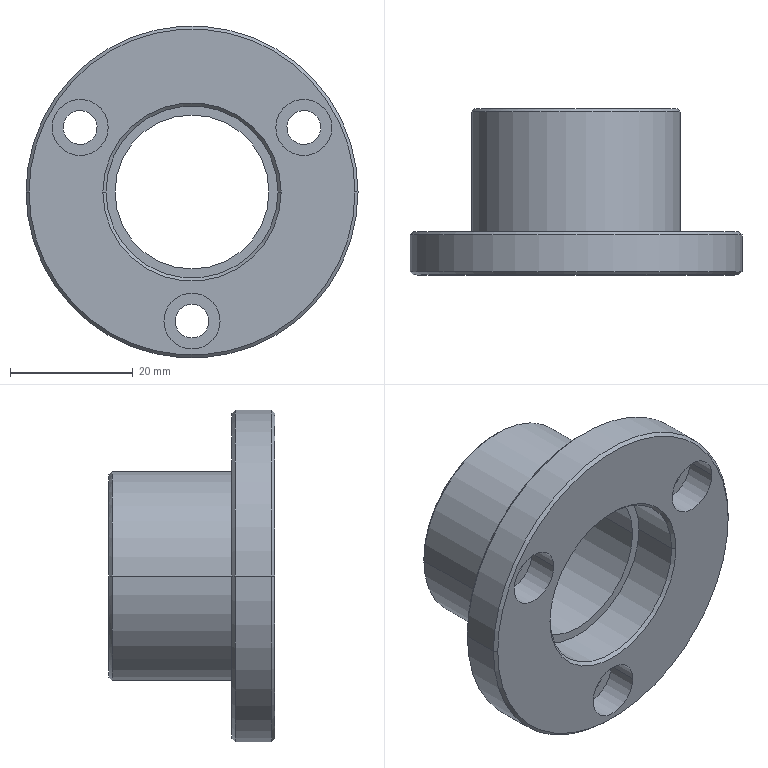Part | Creo | features CUT 4, CURVE 3, DATUM PLANE 3, CHAMFER 1, COORDINATE SYSTEM 1, PATTERN 1, PROTRUSION 1 | 1 solid | 40 faces | box 54 x 27 x 54 mm | volume 17717 mm3 | cylinder 22 | cone 10 | plane 8 | commonest cylinder face diameters 5.5 x6 9.13 x6 28 x4 25.045 x2 34 x2 54 x2
STEP:
#1=CARTESIAN_POINT('',(0.,0.,0.));
#2=DIRECTION('',(0.,0.,1.));
#3=DIRECTION('',(1.,0.,0.));
#4=AXIS2_PLACEMENT_3D('',#1,#2,#3);
#5=CARTESIAN_POINT('',(14.,0.5,0.));
#6=VERTEX_POINT('',#5);
#7=CARTESIAN_POINT('',(-14.,0.5,0.));
#8=VERTEX_POINT('',#7);
#9=CARTESIAN_POINT('',(0.,0.5,0.));
#10=DIRECTION('',(0.,1.,0.));
#11=DIRECTION('',(1.,0.,0.));
#12=AXIS2_PLACEMENT_3D('',#9,#10,#11);
#13=CIRCLE('',#12,14.);
#14=EDGE_CURVE('',#6,#8,#13,.T.);
#15=ORIENTED_EDGE('',*,*,#14,.T.);
#16=CARTESIAN_POINT('',(-14.,8.,0.));
#17=VERTEX_POINT('',#16);
#18=CARTESIAN_POINT('',(-14.,8.,0.));
#19=DIRECTION('',(0.,-1.,0.000000001));
#20=VECTOR('',#19,7.5);
#21=LINE('',#18,#20);
#22=EDGE_CURVE('',#17,#8,#21,.T.);
#23=ORIENTED_EDGE('',*,*,#22,.F.);
#24=CARTESIAN_POINT('',(14.,8.,0.));
#25=VERTEX_POINT('',#24);
#26=CARTESIAN_POINT('',(0.,8.,0.));
#27=DIRECTION('',(0.,1.,0.));
#28=DIRECTION('',(1.,0.,0.));
#29=AXIS2_PLACEMENT_3D('',#26,#27,#28);
#30=CIRCLE('',#29,14.);
#31=EDGE_CURVE('',#25,#17,#30,.T.);
#32=ORIENTED_EDGE('',*,*,#31,.F.);
#33=CARTESIAN_POINT('',(14.,8.,0.));
#34=DIRECTION('',(0.,-1.,-0.000000001));
#35=VECTOR('',#34,7.5);
#36=LINE('',#33,#35);
#37=EDGE_CURVE('',#25,#6,#36,.T.);
#38=ORIENTED_EDGE('',*,*,#37,.T.);
#39=EDGE_LOOP('',(#15,#23,#32,#38));
#40=FACE_OUTER_BOUND('',#39,.F.);
#41=CARTESIAN_POINT('',(0.,0.,0.));
#42=DIRECTION('',(0.,1.,0.));
#43=DIRECTION('',(1.,0.,0.));
#44=AXIS2_PLACEMENT_3D('',#41,#42,#43);
#45=CYLINDRICAL_SURFACE('',#44,14.);
#46=ADVANCED_FACE('',(#40),#45,.F.);
#47=CARTESIAN_POINT('',(14.5,0.,0.));
#48=VERTEX_POINT('',#47);
#49=CARTESIAN_POINT('',(-14.5,0.,0.));
#50=VERTEX_POINT('',#49);
#51=CARTESIAN_POINT('',(0.,0.,0.));
#52=DIRECTION('',(0.,1.,0.));
#53=DIRECTION('',(1.,0.,0.));
#54=AXIS2_PLACEMENT_3D('',#51,#52,#53);
#55=CIRCLE('',#54,14.5);
#56=EDGE_CURVE('',#48,#50,#55,.T.);
#57=ORIENTED_EDGE('',*,*,#56,.T.);
#58=CARTESIAN_POINT('',(-14.5,0.000000001,0.000000008));
#59=DIRECTION('',(0.7071,0.7071,-0.000000003));
#60=VECTOR('',#59,0.7071);
#61=LINE('',#58,#60);
#62=EDGE_CURVE('',#50,#8,#61,.T.);
#63=ORIENTED_EDGE('',*,*,#62,.T.);
#64=ORIENTED_EDGE('',*,*,#14,.F.);
#65=CARTESIAN_POINT('',(14.5,0.000000001,-0.000000008));
#66=DIRECTION('',(-0.7071,0.7071,0.000000003));
#67=VECTOR('',#66,0.7071);
#68=LINE('',#65,#67);
#69=EDGE_CURVE('',#48,#6,#68,.T.);
#70=ORIENTED_EDGE('',*,*,#69,.F.);
#71=EDGE_LOOP('',(#57,#63,#64,#70));
#72=FACE_OUTER_BOUND('',#71,.F.);
#73=CARTESIAN_POINT('',(0.,0.25,0.));
#74=DIRECTION('',(0.,-1.,0.));
#75=DIRECTION('',(0.,0.,-1.));
#76=AXIS2_PLACEMENT_3D('',#73,#74,#75);
#77=CONICAL_SURFACE('',#76,14.25,45.);
#78=ADVANCED_FACE('',(#72),#77,.F.);
#79=CARTESIAN_POINT('',(-26.5,0.,0.));
#80=VERTEX_POINT('',#79);
#81=CARTESIAN_POINT('',(26.5,0.,0.));
#82=VERTEX_POINT('',#81);
#83=CARTESIAN_POINT('',(0.,0.,0.));
#84=DIRECTION('',(0.,1.,0.));
#85=DIRECTION('',(-1.,0.,0.));
#86=AXIS2_PLACEMENT_3D('',#83,#84,#85);
#87=CIRCLE('',#86,26.5);
#88=EDGE_CURVE('',#80,#82,#87,.T.);
#89=ORIENTED_EDGE('',*,*,#88,.T.);
#90=CARTESIAN_POINT('',(0.,0.,0.));
#91=DIRECTION('',(0.,1.,0.));
#92=DIRECTION('',(1.,0.,0.));
#93=AXIS2_PLACEMENT_3D('',#90,#91,#92);
#94=CIRCLE('',#93,26.5);
#95=EDGE_CURVE('',#82,#80,#94,.T.);
#96=ORIENTED_EDGE('',*,*,#95,.T.);
#97=EDGE_LOOP('',(#89,#96));
#98=FACE_OUTER_BOUND('',#97,.F.);
#99=CARTESIAN_POINT('',(13.622,0.,10.5));
#100=VERTEX_POINT('',#99);
#101=CARTESIAN_POINT('',(22.751,0.,10.5));
#102=VERTEX_POINT('',#101);
#103=CARTESIAN_POINT('',(18.187,0.,10.5));
#104=DIRECTION('',(0.,-1.,0.));
#105=DIRECTION('',(-1.,0.,0.));
#106=AXIS2_PLACEMENT_3D('',#103,#104,#105);
#107=CIRCLE('',#106,4.565);
#108=EDGE_CURVE('',#100,#102,#107,.T.);
#109=ORIENTED_EDGE('',*,*,#108,.T.);
#110=CARTESIAN_POINT('',(18.187,0.,10.5));
#111=DIRECTION('',(0.,-1.,0.));
#112=DIRECTION('',(1.,0.,0.));
#113=AXIS2_PLACEMENT_3D('',#110,#111,#112);
#114=CIRCLE('',#113,4.565);
#115=EDGE_CURVE('',#102,#100,#114,.T.);
#116=ORIENTED_EDGE('',*,*,#115,.T.);
#117=EDGE_LOOP('',(#109,#116));
#118=FACE_BOUND('',#117,.F.);
#119=CARTESIAN_POINT('',(-22.751,0.,10.5));
#120=VERTEX_POINT('',#119);
#121=CARTESIAN_POINT('',(-13.622,0.,10.5));
#122=VERTEX_POINT('',#121);
#123=CARTESIAN_POINT('',(-18.187,0.,10.5));
#124=DIRECTION('',(0.,-1.,0.));
#125=DIRECTION('',(-1.,0.,0.));
#126=AXIS2_PLACEMENT_3D('',#123,#124,#125);
#127=CIRCLE('',#126,4.565);
#128=EDGE_CURVE('',#120,#122,#127,.T.);
#129=ORIENTED_EDGE('',*,*,#128,.T.);
#130=CARTESIAN_POINT('',(-18.187,0.,10.5));
#131=DIRECTION('',(0.,-1.,0.));
#132=DIRECTION('',(1.,0.,0.));
#133=AXIS2_PLACEMENT_3D('',#130,#131,#132);
#134=CIRCLE('',#133,4.565);
#135=EDGE_CURVE('',#122,#120,#134,.T.);
#136=ORIENTED_EDGE('',*,*,#135,.T.);
#137=EDGE_LOOP('',(#129,#136));
#138=FACE_BOUND('',#137,.F.);
#139=CARTESIAN_POINT('',(-4.565,0.,-21.));
#140=VERTEX_POINT('',#139);
#141=CARTESIAN_POINT('',(4.565,0.,-21.));
#142=VERTEX_POINT('',#141);
#143=CARTESIAN_POINT('',(0.,0.,-21.));
#144=DIRECTION('',(0.,-1.,0.));
#145=DIRECTION('',(-1.,0.,0.));
#146=AXIS2_PLACEMENT_3D('',#143,#144,#145);
#147=CIRCLE('',#146,4.565);
#148=EDGE_CURVE('',#140,#142,#147,.T.);
#149=ORIENTED_EDGE('',*,*,#148,.T.);
#150=CARTESIAN_POINT('',(0.,0.,-21.));
#151=DIRECTION('',(0.,-1.,0.));
#152=DIRECTION('',(1.,0.,0.));
#153=AXIS2_PLACEMENT_3D('',#150,#151,#152);
#154=CIRCLE('',#153,4.565);
#155=EDGE_CURVE('',#142,#140,#154,.T.);
#156=ORIENTED_EDGE('',*,*,#155,.T.);
#157=EDGE_LOOP('',(#149,#156));
#158=FACE_BOUND('',#157,.F.);
#159=CARTESIAN_POINT('',(0.,0.,0.));
#160=DIRECTION('',(0.,1.,0.));
#161=DIRECTION('',(-1.,0.,0.));
#162=AXIS2_PLACEMENT_3D('',#159,#160,#161);
#163=CIRCLE('',#162,14.5);
#164=EDGE_CURVE('',#50,#48,#163,.T.);
#165=ORIENTED_EDGE('',*,*,#164,.F.);
#166=ORIENTED_EDGE('',*,*,#56,.F.);
#167=EDGE_LOOP('',(#165,#166));
#168=FACE_BOUND('',#167,.F.);
#169=CARTESIAN_POINT('',(0.,0.,0.));
#170=DIRECTION('',(0.,1.,0.));
#171=DIRECTION('',(1.,0.,0.));
#172=AXIS2_PLACEMENT_3D('',#169,#170,#171);
#173=PLANE('',#172);
#174=ADVANCED_FACE('',(#98,#118,#138,#158,#168),#173,.F.);
#175=ORIENTED_EDGE('',*,*,#148,.F.);
#176=CARTESIAN_POINT('',(-4.565,5.,-21.));
#177=VERTEX_POINT('',#176);
#178=CARTESIAN_POINT('',(-4.565,0.,-21.));
#179=DIRECTION('',(0.,1.,0.));
#180=VECTOR('',#179,5.);
#181=LINE('',#178,#180);
#182=EDGE_CURVE('',#140,#177,#181,.T.);
#183=ORIENTED_EDGE('',*,*,#182,.T.);
#184=CARTESIAN_POINT('',(4.565,5.,-21.));
#185=VERTEX_POINT('',#184);
#186=CARTESIAN_POINT('',(0.,5.,-21.));
#187=DIRECTION('',(0.,-1.,0.));
#188=DIRECTION('',(-1.,0.,0.));
#189=AXIS2_PLACEMENT_3D('',#186,#187,#188);
#190=CIRCLE('',#189,4.565);
#191=EDGE_CURVE('',#177,#185,#190,.T.);
#192=ORIENTED_EDGE('',*,*,#191,.T.);
#193=CARTESIAN_POINT('',(4.565,0.,-21.));
#194=DIRECTION('',(0.,1.,0.));
#195=VECTOR('',#194,5.);
#196=LINE('',#193,#195);
#197=EDGE_CURVE('',#142,#185,#196,.T.);
#198=ORIENTED_EDGE('',*,*,#197,.F.);
#199=EDGE_LOOP('',(#175,#183,#192,#198));
#200=FACE_OUTER_BOUND('',#199,.F.);
#201=CARTESIAN_POINT('',(0.,0.,-21.));
#202=DIRECTION('',(0.,-1.,0.));
#203=DIRECTION('',(-1.,0.,0.));
#204=AXIS2_PLACEMENT_3D('',#201,#202,#203);
#205=CYLINDRICAL_SURFACE('',#204,4.565);
#206=ADVANCED_FACE('',(#200),#205,.F.);
#207=ORIENTED_EDGE('',*,*,#155,.F.);
#208=ORIENTED_EDGE('',*,*,#197,.T.);
#209=CARTESIAN_POINT('',(0.,5.,-21.));
#210=DIRECTION('',(0.,-1.,0.));
#211=DIRECTION('',(1.,0.,0.));
#212=AXIS2_PLACEMENT_3D('',#209,#210,#211);
#213=CIRCLE('',#212,4.565);
#214=EDGE_CURVE('',#185,#177,#213,.T.);
#215=ORIENTED_EDGE('',*,*,#214,.T.);
#216=ORIENTED_EDGE('',*,*,#182,.F.);
#217=EDGE_LOOP('',(#207,#208,#215,#216));
#218=FACE_OUTER_BOUND('',#217,.F.);
#219=CARTESIAN_POINT('',(0.,0.,-21.));
#220=DIRECTION('',(0.,-1.,0.));
#221=DIRECTION('',(-1.,0.,0.));
#222=AXIS2_PLACEMENT_3D('',#219,#220,#221);
#223=CYLINDRICAL_SURFACE('',#222,4.565);
#224=ADVANCED_FACE('',(#218),#223,.F.);
#225=ORIENTED_EDGE('',*,*,#191,.F.);
#226=ORIENTED_EDGE('',*,*,#214,.F.);
#227=EDGE_LOOP('',(#225,#226));
#228=FACE_OUTER_BOUND('',#227,.F.);
#229=CARTESIAN_POINT('',(2.75,5.,-21.));
#230=VERTEX_POINT('',#229);
#231=CARTESIAN_POINT('',(-2.75,5.,-21.));
#232=VERTEX_POINT('',#231);
#233=CARTESIAN_POINT('',(0.,5.,-21.));
#234=DIRECTION('',(0.,1.,0.));
#235=DIRECTION('',(1.,0.,0.));
#236=AXIS2_PLACEMENT_3D('',#233,#234,#235);
#237=CIRCLE('',#236,2.75);
#238=EDGE_CURVE('',#230,#232,#237,.T.);
#239=ORIENTED_EDGE('',*,*,#238,.F.);
#240=CARTESIAN_POINT('',(0.,5.,-21.));
#241=DIRECTION('',(0.,1.,0.));
#242=DIRECTION('',(-1.,0.,0.));
#243=AXIS2_PLACEMENT_3D('',#240,#241,#242);
#244=CIRCLE('',#243,2.75);
#245=EDGE_CURVE('',#232,#230,#244,.T.);
#246=ORIENTED_EDGE('',*,*,#245,.F.);
#247=EDGE_LOOP('',(#239,#246));
#248=FACE_BOUND('',#247,.F.);
#249=CARTESIAN_POINT('',(0.,5.,0.));
#250=DIRECTION('',(0.,-1.,0.));
#251=DIRECTION('',(-1.,0.,0.));
#252=AXIS2_PLACEMENT_3D('',#249,#250,#251);
#253=PLANE('',#252);
#254=ADVANCED_FACE('',(#228,#248),#253,.T.);
#255=CARTESIAN_POINT('',(13.622,5.,10.5));
#256=VERTEX_POINT('',#255);
#257=CARTESIAN_POINT('',(22.751,5.,10.5));
#258=VERTEX_POINT('',#257);
#259=CARTESIAN_POINT('',(18.187,5.,10.5));
#260=DIRECTION('',(0.,-1.,0.));
#261=DIRECTION('',(-1.,0.,0.));
#262=AXIS2_PLACEMENT_3D('',#259,#260,#261);
#263=CIRCLE('',#262,4.565);
#264=EDGE_CURVE('',#256,#258,#263,.T.);
#265=ORIENTED_EDGE('',*,*,#264,.F.);
#266=CARTESIAN_POINT('',(18.187,5.,10.5));
#267=DIRECTION('',(0.,-1.,0.));
#268=DIRECTION('',(1.,0.,0.));
#269=AXIS2_PLACEMENT_3D('',#266,#267,#268);
#270=CIRCLE('',#269,4.565);
#271=EDGE_CURVE('',#258,#256,#270,.T.);
#272=ORIENTED_EDGE('',*,*,#271,.F.);
#273=EDGE_LOOP('',(#265,#272));
#274=FACE_OUTER_BOUND('',#273,.F.);
#275=CARTESIAN_POINT('',(16.812,5.,12.882));
#276=VERTEX_POINT('',#275);
#277=CARTESIAN_POINT('',(19.562,5.,8.118));
#278=VERTEX_POINT('',#277);
#279=CARTESIAN_POINT('',(18.187,5.,10.5));
#280=DIRECTION('',(0.,1.,0.));
#281=DIRECTION('',(-0.5,0.,0.866));
#282=AXIS2_PLACEMENT_3D('',#279,#280,#281);
#283=CIRCLE('',#282,2.75);
#284=EDGE_CURVE('',#276,#278,#283,.T.);
#285=ORIENTED_EDGE('',*,*,#284,.F.);
#286=CARTESIAN_POINT('',(18.187,5.,10.5));
#287=DIRECTION('',(0.,1.,0.));
#288=DIRECTION('',(0.5,0.,-0.866));
#289=AXIS2_PLACEMENT_3D('',#286,#287,#288);
#290=CIRCLE('',#289,2.75);
#291=EDGE_CURVE('',#278,#276,#290,.T.);
#292=ORIENTED_EDGE('',*,*,#291,.F.);
#293=EDGE_LOOP('',(#285,#292));
#294=FACE_BOUND('',#293,.F.);
#295=CARTESIAN_POINT('',(0.,5.,0.));
#296=DIRECTION('',(0.,-1.,0.));
#297=DIRECTION('',(-1.,0.,0.));
#298=AXIS2_PLACEMENT_3D('',#295,#296,#297);
#299=PLANE('',#298);
#300=ADVANCED_FACE('',(#274,#294),#299,.T.);
#301=CARTESIAN_POINT('',(-22.751,5.,10.5));
#302=VERTEX_POINT('',#301);
#303=CARTESIAN_POINT('',(-13.622,5.,10.5));
#304=VERTEX_POINT('',#303);
#305=CARTESIAN_POINT('',(-18.187,5.,10.5));
#306=DIRECTION('',(0.,-1.,0.));
#307=DIRECTION('',(-1.,0.,0.));
#308=AXIS2_PLACEMENT_3D('',#305,#306,#307);
#309=CIRCLE('',#308,4.565);
#310=EDGE_CURVE('',#302,#304,#309,.T.);
#311=ORIENTED_EDGE('',*,*,#310,.F.);
#312=CARTESIAN_POINT('',(-18.187,5.,10.5));
#313=DIRECTION('',(0.,-1.,0.));
#314=DIRECTION('',(1.,0.,0.));
#315=AXIS2_PLACEMENT_3D('',#312,#313,#314);
#316=CIRCLE('',#315,4.565);
#317=EDGE_CURVE('',#304,#302,#316,.T.);
#318=ORIENTED_EDGE('',*,*,#317,.F.);
#319=EDGE_LOOP('',(#311,#318));
#320=FACE_OUTER_BOUND('',#319,.F.);
#321=CARTESIAN_POINT('',(-19.562,5.,8.118));
#322=VERTEX_POINT('',#321);
#323=CARTESIAN_POINT('',(-16.812,5.,12.882));
#324=VERTEX_POINT('',#323);
#325=CARTESIAN_POINT('',(-18.187,5.,10.5));
#326=DIRECTION('',(0.,1.,0.));
#327=DIRECTION('',(-0.5,0.,-0.866));
#328=AXIS2_PLACEMENT_3D('',#325,#326,#327);
#329=CIRCLE('',#328,2.75);
#330=EDGE_CURVE('',#322,#324,#329,.T.);
#331=ORIENTED_EDGE('',*,*,#330,.F.);
#332=CARTESIAN_POINT('',(-18.187,5.,10.5));
#333=DIRECTION('',(0.,1.,0.));
#334=DIRECTION('',(0.5,0.,0.866));
#335=AXIS2_PLACEMENT_3D('',#332,#333,#334);
#336=CIRCLE('',#335,2.75);
#337=EDGE_CURVE('',#324,#322,#336,.T.);
#338=ORIENTED_EDGE('',*,*,#337,.F.);
#339=EDGE_LOOP('',(#331,#338));
#340=FACE_BOUND('',#339,.F.);
#341=CARTESIAN_POINT('',(0.,5.,0.));
#342=DIRECTION('',(0.,-1.,0.));
#343=DIRECTION('',(-1.,0.,0.));
#344=AXIS2_PLACEMENT_3D('',#341,#342,#343);
#345=PLANE('',#344);
#346=ADVANCED_FACE('',(#320,#340),#345,.T.);
#347=ORIENTED_EDGE('',*,*,#108,.F.);
#348=CARTESIAN_POINT('',(13.622,0.,10.5));
#349=DIRECTION('',(0.,1.,0.));
#350=VECTOR('',#349,5.);
#351=LINE('',#348,#350);
#352=EDGE_CURVE('',#100,#256,#351,.T.);
#353=ORIENTED_EDGE('',*,*,#352,.T.);
#354=ORIENTED_EDGE('',*,*,#264,.T.);
#355=CARTESIAN_POINT('',(22.751,0.,10.5));
#356=DIRECTION('',(0.,1.,0.));
#357=VECTOR('',#356,5.);
#358=LINE('',#355,#357);
#359=EDGE_CURVE('',#102,#258,#358,.T.);
#360=ORIENTED_EDGE('',*,*,#359,.F.);
#361=EDGE_LOOP('',(#347,#353,#354,#360));
#362=FACE_OUTER_BOUND('',#361,.F.);
#363=CARTESIAN_POINT('',(18.187,0.,10.5));
#364=DIRECTION('',(0.,-1.,0.));
#365=DIRECTION('',(-1.,0.,0.));
#366=AXIS2_PLACEMENT_3D('',#363,#364,#365);
#367=CYLINDRICAL_SURFACE('',#366,4.565);
#368=ADVANCED_FACE('',(#362),#367,.F.);
#369=ORIENTED_EDGE('',*,*,#115,.F.);
#370=ORIENTED_EDGE('',*,*,#359,.T.);
#371=ORIENTED_EDGE('',*,*,#271,.T.);
#372=ORIENTED_EDGE('',*,*,#352,.F.);
#373=EDGE_LOOP('',(#369,#370,#371,#372));
#374=FACE_OUTER_BOUND('',#373,.F.);
#375=CARTESIAN_POINT('',(18.187,0.,10.5));
#376=DIRECTION('',(0.,-1.,0.));
#377=DIRECTION('',(-1.,0.,0.));
#378=AXIS2_PLACEMENT_3D('',#375,#376,#377);
#379=CYLINDRICAL_SURFACE('',#378,4.565);
#380=ADVANCED_FACE('',(#374),#379,.F.);
#381=ORIENTED_EDGE('',*,*,#128,.F.);
#382=CARTESIAN_POINT('',(-22.751,0.,10.5));
#383=DIRECTION('',(0.,1.,0.));
#384=VECTOR('',#383,5.);
#385=LINE('',#382,#384);
#386=EDGE_CURVE('',#120,#302,#385,.T.);
#387=ORIENTED_EDGE('',*,*,#386,.T.);
#388=ORIENTED_EDGE('',*,*,#310,.T.);
#389=CARTESIAN_POINT('',(-13.622,0.,10.5));
#390=DIRECTION('',(0.,1.,0.));
#391=VECTOR('',#390,5.);
#392=LINE('',#389,#391);
#393=EDGE_CURVE('',#122,#304,#392,.T.);
#394=ORIENTED_EDGE('',*,*,#393,.F.);
#395=EDGE_LOOP('',(#381,#387,#388,#394));
#396=FACE_OUTER_BOUND('',#395,.F.);
#397=CARTESIAN_POINT('',(-18.187,0.,10.5));
#398=DIRECTION('',(0.,-1.,0.));
#399=DIRECTION('',(-1.,0.,0.));
#400=AXIS2_PLACEMENT_3D('',#397,#398,#399);
#401=CYLINDRICAL_SURFACE('',#400,4.565);
#402=ADVANCED_FACE('',(#396),#401,.F.);
#403=ORIENTED_EDGE('',*,*,#135,.F.);
#404=ORIENTED_EDGE('',*,*,#393,.T.);
#405=ORIENTED_EDGE('',*,*,#317,.T.);
#406=ORIENTED_EDGE('',*,*,#386,.F.);
#407=EDGE_LOOP('',(#403,#404,#405,#406));
#408=FACE_OUTER_BOUND('',#407,.F.);
#409=CARTESIAN_POINT('',(-18.187,0.,10.5));
#410=DIRECTION('',(0.,-1.,0.));
#411=DIRECTION('',(-1.,0.,0.));
#412=AXIS2_PLACEMENT_3D('',#409,#410,#411);
#413=CYLINDRICAL_SURFACE('',#412,4.565);
#414=ADVANCED_FACE('',(#408),#413,.F.);
#415=ORIENTED_EDGE('',*,*,#238,.T.);
#416=CARTESIAN_POINT('',(-2.75,7.,-21.));
#417=VERTEX_POINT('',#416);
#418=CARTESIAN_POINT('',(-2.75,7.,-21.));
#419=DIRECTION('',(0.,-1.,0.));
#420=VECTOR('',#419,2.);
#421=LINE('',#418,#420);
#422=EDGE_CURVE('',#417,#232,#421,.T.);
#423=ORIENTED_EDGE('',*,*,#422,.F.);
#424=CARTESIAN_POINT('',(2.75,7.,-21.));
#425=VERTEX_POINT('',#424);
#426=CARTESIAN_POINT('',(0.,7.,-21.));
#427=DIRECTION('',(0.,1.,0.));
#428=DIRECTION('',(1.,0.,0.));
#429=AXIS2_PLACEMENT_3D('',#426,#427,#428);
#430=CIRCLE('',#429,2.75);
#431=EDGE_CURVE('',#425,#417,#430,.T.);
#432=ORIENTED_EDGE('',*,*,#431,.F.);
#433=CARTESIAN_POINT('',(2.75,7.,-21.));
#434=DIRECTION('',(0.,-1.,0.));
#435=VECTOR('',#434,2.);
#436=LINE('',#433,#435);
#437=EDGE_CURVE('',#425,#230,#436,.T.);
#438=ORIENTED_EDGE('',*,*,#437,.T.);
#439=EDGE_LOOP('',(#415,#423,#432,#438));
#440=FACE_OUTER_BOUND('',#439,.F.);
#441=CARTESIAN_POINT('',(0.,7.,-21.));
#442=DIRECTION('',(0.,1.,0.));
#443=DIRECTION('',(1.,0.,0.));
#444=AXIS2_PLACEMENT_3D('',#441,#442,#443);
#445=CYLINDRICAL_SURFACE('',#444,2.75);
#446=ADVANCED_FACE('',(#440),#445,.F.);
#447=ORIENTED_EDGE('',*,*,#245,.T.);
#448=ORIENTED_EDGE('',*,*,#437,.F.);
#449=CARTESIAN_POINT('',(0.,7.,-21.));
#450=DIRECTION('',(0.,1.,0.));
#451=DIRECTION('',(-1.,0.,0.));
#452=AXIS2_PLACEMENT_3D('',#449,#450,#451);
#453=CIRCLE('',#452,2.75);
#454=EDGE_CURVE('',#417,#425,#453,.T.);
#455=ORIENTED_EDGE('',*,*,#454,.F.);
#456=ORIENTED_EDGE('',*,*,#422,.T.);
#457=EDGE_LOOP('',(#447,#448,#455,#456));
#458=FACE_OUTER_BOUND('',#457,.F.);
#459=CARTESIAN_POINT('',(0.,7.,-21.));
#460=DIRECTION('',(0.,1.,0.));
#461=DIRECTION('',(1.,0.,0.));
#462=AXIS2_PLACEMENT_3D('',#459,#460,#461);
#463=CYLINDRICAL_SURFACE('',#462,2.75);
#464=ADVANCED_FACE('',(#458),#463,.F.);
#465=CARTESIAN_POINT('',(-26.5,7.,0.));
#466=VERTEX_POINT('',#465);
#467=CARTESIAN_POINT('',(26.5,7.,0.));
#468=VERTEX_POINT('',#467);
#469=CARTESIAN_POINT('',(0.,7.,0.));
#470=DIRECTION('',(0.,1.,0.));
#471=DIRECTION('',(-1.,0.,0.));
#472=AXIS2_PLACEMENT_3D('',#469,#470,#471);
#473=CIRCLE('',#472,26.5);
#474=EDGE_CURVE('',#466,#468,#473,.T.);
#475=ORIENTED_EDGE('',*,*,#474,.F.);
#476=CARTESIAN_POINT('',(0.,7.,0.));
#477=DIRECTION('',(0.,1.,0.));
#478=DIRECTION('',(1.,0.,0.));
#479=AXIS2_PLACEMENT_3D('',#476,#477,#478);
#480=CIRCLE('',#479,26.5);
#481=EDGE_CURVE('',#468,#466,#480,.T.);
#482=ORIENTED_EDGE('',*,*,#481,.F.);
#483=EDGE_LOOP('',(#475,#482));
#484=FACE_OUTER_BOUND('',#483,.F.);
#485=ORIENTED_EDGE('',*,*,#431,.T.);
#486=ORIENTED_EDGE('',*,*,#454,.T.);
#487=EDGE_LOOP('',(#485,#486));
#488=FACE_BOUND('',#487,.F.);
#489=CARTESIAN_POINT('',(-19.562,7.,8.118));
#490=VERTEX_POINT('',#489);
#491=CARTESIAN_POINT('',(-16.812,7.,12.882));
#492=VERTEX_POINT('',#491);
#493=CARTESIAN_POINT('',(-18.187,7.,10.5));
#494=DIRECTION('',(0.,1.,0.));
#495=DIRECTION('',(-0.5,0.,-0.866));
#496=AXIS2_PLACEMENT_3D('',#493,#494,#495);
#497=CIRCLE('',#496,2.75);
#498=EDGE_CURVE('',#490,#492,#497,.T.);
#499=ORIENTED_EDGE('',*,*,#498,.T.);
#500=CARTESIAN_POINT('',(-18.187,7.,10.5));
#501=DIRECTION('',(0.,1.,0.));
#502=DIRECTION('',(0.5,0.,0.866));
#503=AXIS2_PLACEMENT_3D('',#500,#501,#502);
#504=CIRCLE('',#503,2.75);
#505=EDGE_CURVE('',#492,#490,#504,.T.);
#506=ORIENTED_EDGE('',*,*,#505,.T.);
#507=EDGE_LOOP('',(#499,#506));
#508=FACE_BOUND('',#507,.F.);
#509=CARTESIAN_POINT('',(16.812,7.,12.882));
#510=VERTEX_POINT('',#509);
#511=CARTESIAN_POINT('',(19.562,7.,8.118));
#512=VERTEX_POINT('',#511);
#513=CARTESIAN_POINT('',(18.187,7.,10.5));
#514=DIRECTION('',(0.,1.,0.));
#515=DIRECTION('',(-0.5,0.,0.866));
#516=AXIS2_PLACEMENT_3D('',#513,#514,#515);
#517=CIRCLE('',#516,2.75);
#518=EDGE_CURVE('',#510,#512,#517,.T.);
#519=ORIENTED_EDGE('',*,*,#518,.T.);
#520=CARTESIAN_POINT('',(18.187,7.,10.5));
#521=DIRECTION('',(0.,1.,0.));
#522=DIRECTION('',(0.5,0.,-0.866));
#523=AXIS2_PLACEMENT_3D('',#520,#521,#522);
#524=CIRCLE('',#523,2.75);
#525=EDGE_CURVE('',#512,#510,#524,.T.);
#526=ORIENTED_EDGE('',*,*,#525,.T.);
#527=EDGE_LOOP('',(#519,#526));
#528=FACE_BOUND('',#527,.F.);
#529=CARTESIAN_POINT('',(17.,7.,0.));
#530=VERTEX_POINT('',#529);
#531=CARTESIAN_POINT('',(-17.,7.,0.));
#532=VERTEX_POINT('',#531);
#533=CARTESIAN_POINT('',(0.,7.,0.));
#534=DIRECTION('',(0.,-1.,0.));
#535=DIRECTION('',(1.,0.,0.));
#536=AXIS2_PLACEMENT_3D('',#533,#534,#535);
#537=CIRCLE('',#536,17.);
#538=EDGE_CURVE('',#530,#532,#537,.T.);
#539=ORIENTED_EDGE('',*,*,#538,.F.);
#540=CARTESIAN_POINT('',(0.,7.,0.));
#541=DIRECTION('',(0.,1.,0.));
#542=DIRECTION('',(1.,0.,0.));
#543=AXIS2_PLACEMENT_3D('',#540,#541,#542);
#544=CIRCLE('',#543,17.);
#545=EDGE_CURVE('',#530,#532,#544,.T.);
#546=ORIENTED_EDGE('',*,*,#545,.T.);
#547=EDGE_LOOP('',(#539,#546));
#548=FACE_BOUND('',#547,.F.);
#549=CARTESIAN_POINT('',(0.,7.,0.));
#550=DIRECTION('',(0.,1.,0.));
#551=DIRECTION('',(1.,0.,0.));
#552=AXIS2_PLACEMENT_3D('',#549,#550,#551);
#553=PLANE('',#552);
#554=ADVANCED_FACE('',(#484,#488,#508,#528,#548),#553,.T.);
#555=CARTESIAN_POINT('',(-17.,26.5,0.));
#556=VERTEX_POINT('',#555);
#557=CARTESIAN_POINT('',(17.,26.5,0.));
#558=VERTEX_POINT('',#557);
#559=CARTESIAN_POINT('',(0.,26.5,0.));
#560=DIRECTION('',(0.,1.,0.));
#561=DIRECTION('',(-1.,0.,0.));
#562=AXIS2_PLACEMENT_3D('',#559,#560,#561);
#563=CIRCLE('',#562,17.);
#564=EDGE_CURVE('',#556,#558,#563,.T.);
#565=ORIENTED_EDGE('',*,*,#564,.T.);
#566=CARTESIAN_POINT('',(17.,7.,0.));
#567=DIRECTION('',(0.,1.,0.));
#568=VECTOR('',#567,19.5);
#569=LINE('',#566,#568);
#570=EDGE_CURVE('',#530,#558,#569,.T.);
#571=ORIENTED_EDGE('',*,*,#570,.F.);
#572=ORIENTED_EDGE('',*,*,#538,.T.);
#573=CARTESIAN_POINT('',(-17.,7.,0.));
#574=DIRECTION('',(0.,1.,0.));
#575=VECTOR('',#574,19.5);
#576=LINE('',#573,#575);
#577=EDGE_CURVE('',#532,#556,#576,.T.);
#578=ORIENTED_EDGE('',*,*,#577,.T.);
#579=EDGE_LOOP('',(#565,#571,#572,#578));
#580=FACE_OUTER_BOUND('',#579,.F.);
#581=CARTESIAN_POINT('',(0.,0.,0.));
#582=DIRECTION('',(0.,1.,0.));
#583=DIRECTION('',(1.,0.,0.));
#584=AXIS2_PLACEMENT_3D('',#581,#582,#583);
#585=CYLINDRICAL_SURFACE('',#584,17.);
#586=ADVANCED_FACE('',(#580),#585,.T.);
#587=CARTESIAN_POINT('',(-16.5,27.,0.));
#588=VERTEX_POINT('',#587);
#589=CARTESIAN_POINT('',(16.5,27.,0.));
#590=VERTEX_POINT('',#589);
#591=CARTESIAN_POINT('',(0.,27.,0.));
#592=DIRECTION('',(0.,1.,0.));
#593=DIRECTION('',(-1.,0.,0.));
#594=AXIS2_PLACEMENT_3D('',#591,#592,#593);
#595=CIRCLE('',#594,16.5);
#596=EDGE_CURVE('',#588,#590,#595,.T.);
#597=ORIENTED_EDGE('',*,*,#596,.T.);
#598=CARTESIAN_POINT('',(16.5,27.,-0.000000005));
#599=DIRECTION('',(0.7071,-0.7071,0.000000001));
#600=VECTOR('',#599,0.7071);
#601=LINE('',#598,#600);
#602=EDGE_CURVE('',#590,#558,#601,.T.);
#603=ORIENTED_EDGE('',*,*,#602,.T.);
#604=ORIENTED_EDGE('',*,*,#564,.F.);
#605=CARTESIAN_POINT('',(-16.5,27.,0.000000005));
#606=DIRECTION('',(-0.7071,-0.7071,-0.000000001));
#607=VECTOR('',#606,0.7071);
#608=LINE('',#605,#607);
#609=EDGE_CURVE('',#588,#556,#608,.T.);
#610=ORIENTED_EDGE('',*,*,#609,.F.);
#611=EDGE_LOOP('',(#597,#603,#604,#610));
#612=FACE_OUTER_BOUND('',#611,.F.);
#613=CARTESIAN_POINT('',(0.,26.75,0.));
#614=DIRECTION('',(0.,-1.,0.));
#615=DIRECTION('',(0.,0.,-1.));
#616=AXIS2_PLACEMENT_3D('',#613,#614,#615);
#617=CONICAL_SURFACE('',#616,16.75,45.);
#618=ADVANCED_FACE('',(#612),#617,.T.);
#619=ORIENTED_EDGE('',*,*,#596,.F.);
#620=CARTESIAN_POINT('',(0.,27.,0.));
#621=DIRECTION('',(0.,1.,0.));
#622=DIRECTION('',(1.,0.,0.));
#623=AXIS2_PLACEMENT_3D('',#620,#621,#622);
#624=CIRCLE('',#623,16.5);
#625=EDGE_CURVE('',#590,#588,#624,.T.);
#626=ORIENTED_EDGE('',*,*,#625,.F.);
#627=EDGE_LOOP('',(#619,#626));
#628=FACE_OUTER_BOUND('',#627,.F.);
#629=CARTESIAN_POINT('',(-14.5,27.,0.));
#630=VERTEX_POINT('',#629);
#631=CARTESIAN_POINT('',(14.5,27.,0.));
#632=VERTEX_POINT('',#631);
#633=CARTESIAN_POINT('',(0.,27.,0.));
#634=DIRECTION('',(0.,1.,0.));
#635=DIRECTION('',(-1.,0.,0.));
#636=AXIS2_PLACEMENT_3D('',#633,#634,#635);
#637=CIRCLE('',#636,14.5);
#638=EDGE_CURVE('',#630,#632,#637,.T.);
#639=ORIENTED_EDGE('',*,*,#638,.T.);
#640=CARTESIAN_POINT('',(0.,27.,0.));
#641=DIRECTION('',(0.,1.,0.));
#642=DIRECTION('',(1.,0.,0.));
#643=AXIS2_PLACEMENT_3D('',#640,#641,#642);
#644=CIRCLE('',#643,14.5);
#645=EDGE_CURVE('',#632,#630,#644,.T.);
#646=ORIENTED_EDGE('',*,*,#645,.T.);
#647=EDGE_LOOP('',(#639,#646));
#648=FACE_BOUND('',#647,.F.);
#649=CARTESIAN_POINT('',(0.,27.,0.));
#650=DIRECTION('',(0.,1.,0.));
#651=DIRECTION('',(1.,0.,0.));
#652=AXIS2_PLACEMENT_3D('',#649,#650,#651);
#653=PLANE('',#652);
#654=ADVANCED_FACE('',(#628,#648),#653,.T.);
#655=ORIENTED_EDGE('',*,*,#625,.T.);
#656=ORIENTED_EDGE('',*,*,#609,.T.);
#657=CARTESIAN_POINT('',(0.,26.5,0.));
#658=DIRECTION('',(0.,1.,0.));
#659=DIRECTION('',(1.,0.,0.));
#660=AXIS2_PLACEMENT_3D('',#657,#658,#659);
#661=CIRCLE('',#660,17.);
#662=EDGE_CURVE('',#558,#556,#661,.T.);
#663=ORIENTED_EDGE('',*,*,#662,.F.);
#664=ORIENTED_EDGE('',*,*,#602,.F.);
#665=EDGE_LOOP('',(#655,#656,#663,#664));
#666=FACE_OUTER_BOUND('',#665,.F.);
#667=CARTESIAN_POINT('',(0.,26.75,0.));
#668=DIRECTION('',(0.,-1.,0.));
#669=DIRECTION('',(0.,0.,-1.));
#670=AXIS2_PLACEMENT_3D('',#667,#668,#669);
#671=CONICAL_SURFACE('',#670,16.75,45.);
#672=ADVANCED_FACE('',(#666),#671,.T.);
#673=ORIENTED_EDGE('',*,*,#662,.T.);
#674=ORIENTED_EDGE('',*,*,#577,.F.);
#675=ORIENTED_EDGE('',*,*,#545,.F.);
#676=ORIENTED_EDGE('',*,*,#570,.T.);
#677=EDGE_LOOP('',(#673,#674,#675,#676));
#678=FACE_OUTER_BOUND('',#677,.F.);
#679=CARTESIAN_POINT('',(0.,0.,0.));
#680=DIRECTION('',(0.,1.,0.));
#681=DIRECTION('',(1.,0.,0.));
#682=AXIS2_PLACEMENT_3D('',#679,#680,#681);
#683=CYLINDRICAL_SURFACE('',#682,17.);
#684=ADVANCED_FACE('',(#678),#683,.T.);
#685=CARTESIAN_POINT('',(-14.,26.5,0.));
#686=VERTEX_POINT('',#685);
#687=CARTESIAN_POINT('',(14.,26.5,0.));
#688=VERTEX_POINT('',#687);
#689=CARTESIAN_POINT('',(0.,26.5,0.));
#690=DIRECTION('',(0.,1.,0.));
#691=DIRECTION('',(-1.,0.,0.));
#692=AXIS2_PLACEMENT_3D('',#689,#690,#691);
#693=CIRCLE('',#692,14.);
#694=EDGE_CURVE('',#686,#688,#693,.T.);
#695=ORIENTED_EDGE('',*,*,#694,.T.);
#696=CARTESIAN_POINT('',(14.,26.5,0.000000002));
#697=DIRECTION('',(0.7071,0.7071,0.000000001));
#698=VECTOR('',#697,0.7071);
#699=LINE('',#696,#698);
#700=EDGE_CURVE('',#688,#632,#699,.T.);
#701=ORIENTED_EDGE('',*,*,#700,.T.);
#702=ORIENTED_EDGE('',*,*,#638,.F.);
#703=CARTESIAN_POINT('',(-14.,26.5,-0.000000002));
#704=DIRECTION('',(-0.7071,0.7071,-0.000000001));
#705=VECTOR('',#704,0.7071);
#706=LINE('',#703,#705);
#707=EDGE_CURVE('',#686,#630,#706,.T.);
#708=ORIENTED_EDGE('',*,*,#707,.F.);
#709=EDGE_LOOP('',(#695,#701,#702,#708));
#710=FACE_OUTER_BOUND('',#709,.F.);
#711=CARTESIAN_POINT('',(0.,26.75,0.));
#712=DIRECTION('',(0.,1.,0.));
#713=DIRECTION('',(0.,0.,-1.));
#714=AXIS2_PLACEMENT_3D('',#711,#712,#713);
#715=CONICAL_SURFACE('',#714,14.25,45.);
#716=ADVANCED_FACE('',(#710),#715,.F.);
#717=ORIENTED_EDGE('',*,*,#694,.F.);
#718=CARTESIAN_POINT('',(-14.,19.,0.));
#719=VERTEX_POINT('',#718);
#720=CARTESIAN_POINT('',(-14.,26.5,-0.000000002));
#721=DIRECTION('',(0.,-1.,0.));
#722=VECTOR('',#721,7.5);
#723=LINE('',#720,#722);
#724=EDGE_CURVE('',#686,#719,#723,.T.);
#725=ORIENTED_EDGE('',*,*,#724,.T.);
#726=CARTESIAN_POINT('',(14.,19.,0.));
#727=VERTEX_POINT('',#726);
#728=CARTESIAN_POINT('',(0.,19.,0.));
#729=DIRECTION('',(0.,-1.,0.));
#730=DIRECTION('',(1.,0.,0.));
#731=AXIS2_PLACEMENT_3D('',#728,#729,#730);
#732=CIRCLE('',#731,14.);
#733=EDGE_CURVE('',#727,#719,#732,.T.);
#734=ORIENTED_EDGE('',*,*,#733,.F.);
#735=CARTESIAN_POINT('',(14.,26.5,0.000000002));
#736=DIRECTION('',(0.,-1.,0.));
#737=VECTOR('',#736,7.5);
#738=LINE('',#735,#737);
#739=EDGE_CURVE('',#688,#727,#738,.T.);
#740=ORIENTED_EDGE('',*,*,#739,.F.);
#741=EDGE_LOOP('',(#717,#725,#734,#740));
#742=FACE_OUTER_BOUND('',#741,.F.);
#743=CARTESIAN_POINT('',(0.,0.,0.));
#744=DIRECTION('',(0.,1.,0.));
#745=DIRECTION('',(1.,0.,0.));
#746=AXIS2_PLACEMENT_3D('',#743,#744,#745);
#747=CYLINDRICAL_SURFACE('',#746,14.);
#748=ADVANCED_FACE('',(#742),#747,.F.);
#749=CARTESIAN_POINT('',(0.,26.5,0.));
#750=DIRECTION('',(0.,1.,0.));
#751=DIRECTION('',(1.,0.,0.));
#752=AXIS2_PLACEMENT_3D('',#749,#750,#751);
#753=CIRCLE('',#752,14.);
#754=EDGE_CURVE('',#688,#686,#753,.T.);
#755=ORIENTED_EDGE('',*,*,#754,.F.);
#756=ORIENTED_EDGE('',*,*,#739,.T.);
#757=CARTESIAN_POINT('',(0.,19.,0.));
#758=DIRECTION('',(0.,1.,0.));
#759=DIRECTION('',(1.,0.,0.));
#760=AXIS2_PLACEMENT_3D('',#757,#758,#759);
#761=CIRCLE('',#760,14.);
#762=EDGE_CURVE('',#727,#719,#761,.T.);
#763=ORIENTED_EDGE('',*,*,#762,.T.);
#764=ORIENTED_EDGE('',*,*,#724,.F.);
#765=EDGE_LOOP('',(#755,#756,#763,#764));
#766=FACE_OUTER_BOUND('',#765,.F.);
#767=CARTESIAN_POINT('',(0.,0.,0.));
#768=DIRECTION('',(0.,1.,0.));
#769=DIRECTION('',(1.,0.,0.));
#770=AXIS2_PLACEMENT_3D('',#767,#768,#769);
#771=CYLINDRICAL_SURFACE('',#770,14.);
#772=ADVANCED_FACE('',(#766),#771,.F.);
#773=ORIENTED_EDGE('',*,*,#754,.T.);
#774=ORIENTED_EDGE('',*,*,#707,.T.);
#775=ORIENTED_EDGE('',*,*,#645,.F.);
#776=ORIENTED_EDGE('',*,*,#700,.F.);
#777=EDGE_LOOP('',(#773,#774,#775,#776));
#778=FACE_OUTER_BOUND('',#777,.F.);
#779=CARTESIAN_POINT('',(0.,26.75,0.));
#780=DIRECTION('',(0.,1.,0.));
#781=DIRECTION('',(0.,0.,-1.));
#782=AXIS2_PLACEMENT_3D('',#779,#780,#781);
#783=CONICAL_SURFACE('',#782,14.25,45.);
#784=ADVANCED_FACE('',(#778),#783,.F.);
#785=ORIENTED_EDGE('',*,*,#762,.F.);
#786=ORIENTED_EDGE('',*,*,#733,.T.);
#787=EDGE_LOOP('',(#785,#786));
#788=FACE_OUTER_BOUND('',#787,.F.);
#789=CARTESIAN_POINT('',(12.522,19.,0.));
#790=VERTEX_POINT('',#789);
#791=CARTESIAN_POINT('',(-12.522,19.,0.));
#792=VERTEX_POINT('',#791);
#793=CARTESIAN_POINT('',(0.,19.,0.));
#794=DIRECTION('',(0.,-1.,0.));
#795=DIRECTION('',(1.,0.,0.));
#796=AXIS2_PLACEMENT_3D('',#793,#794,#795);
#797=CIRCLE('',#796,12.522);
#798=EDGE_CURVE('',#790,#792,#797,.T.);
#799=ORIENTED_EDGE('',*,*,#798,.F.);
#800=CARTESIAN_POINT('',(0.,19.,0.));
#801=DIRECTION('',(0.,1.,0.));
#802=DIRECTION('',(1.,0.,0.));
#803=AXIS2_PLACEMENT_3D('',#800,#801,#802);
#804=CIRCLE('',#803,12.522);
#805=EDGE_CURVE('',#790,#792,#804,.T.);
#806=ORIENTED_EDGE('',*,*,#805,.T.);
#807=EDGE_LOOP('',(#799,#806));
#808=FACE_BOUND('',#807,.F.);
#809=CARTESIAN_POINT('',(0.,19.,0.));
#810=DIRECTION('',(0.,1.,0.));
#811=DIRECTION('',(1.,0.,0.));
#812=AXIS2_PLACEMENT_3D('',#809,#810,#811);
#813=PLANE('',#812);
#814=ADVANCED_FACE('',(#788,#808),#813,.T.);
#815=CARTESIAN_POINT('',(12.522,8.,0.));
#816=VERTEX_POINT('',#815);
#817=CARTESIAN_POINT('',(12.522,19.,0.));
#818=DIRECTION('',(0.,-1.,0.));
#819=VECTOR('',#818,11.);
#820=LINE('',#817,#819);
#821=EDGE_CURVE('',#790,#816,#820,.T.);
#822=ORIENTED_EDGE('',*,*,#821,.F.);
#823=ORIENTED_EDGE('',*,*,#798,.T.);
#824=CARTESIAN_POINT('',(-12.522,8.,0.));
#825=VERTEX_POINT('',#824);
#826=CARTESIAN_POINT('',(-12.522,19.,0.));
#827=DIRECTION('',(0.,-1.,0.));
#828=VECTOR('',#827,11.);
#829=LINE('',#826,#828);
#830=EDGE_CURVE('',#792,#825,#829,.T.);
#831=ORIENTED_EDGE('',*,*,#830,.T.);
#832=CARTESIAN_POINT('',(0.,8.,0.));
#833=DIRECTION('',(0.,-1.,0.));
#834=DIRECTION('',(1.,0.,0.));
#835=AXIS2_PLACEMENT_3D('',#832,#833,#834);
#836=CIRCLE('',#835,12.522);
#837=EDGE_CURVE('',#816,#825,#836,.T.);
#838=ORIENTED_EDGE('',*,*,#837,.F.);
#839=EDGE_LOOP('',(#822,#823,#831,#838));
#840=FACE_OUTER_BOUND('',#839,.F.);
#841=CARTESIAN_POINT('',(0.,0.,0.));
#842=DIRECTION('',(0.,1.,0.));
#843=DIRECTION('',(1.,0.,0.));
#844=AXIS2_PLACEMENT_3D('',#841,#842,#843);
#845=CYLINDRICAL_SURFACE('',#844,12.522);
#846=ADVANCED_FACE('',(#840),#845,.F.);
#847=ORIENTED_EDGE('',*,*,#821,.T.);
#848=CARTESIAN_POINT('',(0.,8.,0.));
#849=DIRECTION('',(0.,1.,0.));
#850=DIRECTION('',(1.,0.,0.));
#851=AXIS2_PLACEMENT_3D('',#848,#849,#850);
#852=CIRCLE('',#851,12.522);
#853=EDGE_CURVE('',#816,#825,#852,.T.);
#854=ORIENTED_EDGE('',*,*,#853,.T.);
#855=ORIENTED_EDGE('',*,*,#830,.F.);
#856=ORIENTED_EDGE('',*,*,#805,.F.);
#857=EDGE_LOOP('',(#847,#854,#855,#856));
#858=FACE_OUTER_BOUND('',#857,.F.);
#859=CARTESIAN_POINT('',(0.,0.,0.));
#860=DIRECTION('',(0.,1.,0.));
#861=DIRECTION('',(1.,0.,0.));
#862=AXIS2_PLACEMENT_3D('',#859,#860,#861);
#863=CYLINDRICAL_SURFACE('',#862,12.522);
#864=ADVANCED_FACE('',(#858),#863,.F.);
#865=CARTESIAN_POINT('',(0.,8.,0.));
#866=DIRECTION('',(0.,-1.,0.));
#867=DIRECTION('',(1.,0.,0.));
#868=AXIS2_PLACEMENT_3D('',#865,#866,#867);
#869=CIRCLE('',#868,14.);
#870=EDGE_CURVE('',#25,#17,#869,.T.);
#871=ORIENTED_EDGE('',*,*,#870,.F.);
#872=ORIENTED_EDGE('',*,*,#31,.T.);
#873=EDGE_LOOP('',(#871,#872));
#874=FACE_OUTER_BOUND('',#873,.F.);
#875=ORIENTED_EDGE('',*,*,#853,.F.);
#876=ORIENTED_EDGE('',*,*,#837,.T.);
#877=EDGE_LOOP('',(#875,#876));
#878=FACE_BOUND('',#877,.F.);
#879=CARTESIAN_POINT('',(0.,8.,0.));
#880=DIRECTION('',(0.,1.,0.));
#881=DIRECTION('',(1.,0.,0.));
#882=AXIS2_PLACEMENT_3D('',#879,#880,#881);
#883=PLANE('',#882);
#884=ADVANCED_FACE('',(#874,#878),#883,.F.);
#885=CARTESIAN_POINT('',(0.,0.5,0.));
#886=DIRECTION('',(0.,1.,0.));
#887=DIRECTION('',(-1.,0.,0.));
#888=AXIS2_PLACEMENT_3D('',#885,#886,#887);
#889=CIRCLE('',#888,14.);
#890=EDGE_CURVE('',#8,#6,#889,.T.);
#891=ORIENTED_EDGE('',*,*,#890,.T.);
#892=ORIENTED_EDGE('',*,*,#37,.F.);
#893=ORIENTED_EDGE('',*,*,#870,.T.);
#894=ORIENTED_EDGE('',*,*,#22,.T.);
#895=EDGE_LOOP('',(#891,#892,#893,#894));
#896=FACE_OUTER_BOUND('',#895,.F.);
#897=CARTESIAN_POINT('',(0.,0.,0.));
#898=DIRECTION('',(0.,1.,0.));
#899=DIRECTION('',(1.,0.,0.));
#900=AXIS2_PLACEMENT_3D('',#897,#898,#899);
#901=CYLINDRICAL_SURFACE('',#900,14.);
#902=ADVANCED_FACE('',(#896),#901,.F.);
#903=ORIENTED_EDGE('',*,*,#164,.T.);
#904=ORIENTED_EDGE('',*,*,#69,.T.);
#905=ORIENTED_EDGE('',*,*,#890,.F.);
#906=ORIENTED_EDGE('',*,*,#62,.F.);
#907=EDGE_LOOP('',(#903,#904,#905,#906));
#908=FACE_OUTER_BOUND('',#907,.F.);
#909=CARTESIAN_POINT('',(0.,0.25,0.));
#910=DIRECTION('',(0.,-1.,0.));
#911=DIRECTION('',(0.,0.,-1.));
#912=AXIS2_PLACEMENT_3D('',#909,#910,#911);
#913=CONICAL_SURFACE('',#912,14.25,45.);
#914=ADVANCED_FACE('',(#908),#913,.F.);
#915=ORIENTED_EDGE('',*,*,#330,.T.);
#916=CARTESIAN_POINT('',(-16.812,7.,12.882));
#917=DIRECTION('',(0.,-1.,0.));
#918=VECTOR('',#917,2.);
#919=LINE('',#916,#918);
#920=EDGE_CURVE('',#492,#324,#919,.T.);
#921=ORIENTED_EDGE('',*,*,#920,.F.);
#922=ORIENTED_EDGE('',*,*,#498,.F.);
#923=CARTESIAN_POINT('',(-19.562,7.,8.118));
#924=DIRECTION('',(0.,-1.,0.));
#925=VECTOR('',#924,2.);
#926=LINE('',#923,#925);
#927=EDGE_CURVE('',#490,#322,#926,.T.);
#928=ORIENTED_EDGE('',*,*,#927,.T.);
#929=EDGE_LOOP('',(#915,#921,#922,#928));
#930=FACE_OUTER_BOUND('',#929,.F.);
#931=CARTESIAN_POINT('',(-18.187,7.,10.5));
#932=DIRECTION('',(0.,1.,0.));
#933=DIRECTION('',(-0.5,0.,-0.866));
#934=AXIS2_PLACEMENT_3D('',#931,#932,#933);
#935=CYLINDRICAL_SURFACE('',#934,2.75);
#936=ADVANCED_FACE('',(#930),#935,.F.);
#937=ORIENTED_EDGE('',*,*,#337,.T.);
#938=ORIENTED_EDGE('',*,*,#927,.F.);
#939=ORIENTED_EDGE('',*,*,#505,.F.);
#940=ORIENTED_EDGE('',*,*,#920,.T.);
#941=EDGE_LOOP('',(#937,#938,#939,#940));
#942=FACE_OUTER_BOUND('',#941,.F.);
#943=CARTESIAN_POINT('',(-18.187,7.,10.5));
#944=DIRECTION('',(0.,1.,0.));
#945=DIRECTION('',(-0.5,0.,-0.866));
#946=AXIS2_PLACEMENT_3D('',#943,#944,#945);
#947=CYLINDRICAL_SURFACE('',#946,2.75);
#948=ADVANCED_FACE('',(#942),#947,.F.);
#949=ORIENTED_EDGE('',*,*,#284,.T.);
#950=CARTESIAN_POINT('',(19.562,7.,8.118));
#951=DIRECTION('',(0.,-1.,0.));
#952=VECTOR('',#951,2.);
#953=LINE('',#950,#952);
#954=EDGE_CURVE('',#512,#278,#953,.T.);
#955=ORIENTED_EDGE('',*,*,#954,.F.);
#956=ORIENTED_EDGE('',*,*,#518,.F.);
#957=CARTESIAN_POINT('',(16.812,7.,12.882));
#958=DIRECTION('',(0.,-1.,0.));
#959=VECTOR('',#958,2.);
#960=LINE('',#957,#959);
#961=EDGE_CURVE('',#510,#276,#960,.T.);
#962=ORIENTED_EDGE('',*,*,#961,.T.);
#963=EDGE_LOOP('',(#949,#955,#956,#962));
#964=FACE_OUTER_BOUND('',#963,.F.);
#965=CARTESIAN_POINT('',(18.187,7.,10.5));
#966=DIRECTION('',(0.,1.,0.));
#967=DIRECTION('',(-0.5,0.,0.866));
#968=AXIS2_PLACEMENT_3D('',#965,#966,#967);
#969=CYLINDRICAL_SURFACE('',#968,2.75);
#970=ADVANCED_FACE('',(#964),#969,.F.);
#971=ORIENTED_EDGE('',*,*,#291,.T.);
#972=ORIENTED_EDGE('',*,*,#961,.F.);
#973=ORIENTED_EDGE('',*,*,#525,.F.);
#974=ORIENTED_EDGE('',*,*,#954,.T.);
#975=EDGE_LOOP('',(#971,#972,#973,#974));
#976=FACE_OUTER_BOUND('',#975,.F.);
#977=CARTESIAN_POINT('',(18.187,7.,10.5));
#978=DIRECTION('',(0.,1.,0.));
#979=DIRECTION('',(-0.5,0.,0.866));
#980=AXIS2_PLACEMENT_3D('',#977,#978,#979);
#981=CYLINDRICAL_SURFACE('',#980,2.75);
#982=ADVANCED_FACE('',(#976),#981,.F.);
#983=ORIENTED_EDGE('',*,*,#474,.T.);
#984=CARTESIAN_POINT('',(27.,6.5,0.));
#985=VERTEX_POINT('',#984);
#986=CARTESIAN_POINT('',(26.5,7.,-0.000000004));
#987=DIRECTION('',(0.7071,-0.7071,0.000000001));
#988=VECTOR('',#987,0.7071);
#989=LINE('',#986,#988);
#990=EDGE_CURVE('',#468,#985,#989,.T.);
#991=ORIENTED_EDGE('',*,*,#990,.T.);
#992=CARTESIAN_POINT('',(-27.,6.5,0.));
#993=VERTEX_POINT('',#992);
#994=CARTESIAN_POINT('',(0.,6.5,0.));
#995=DIRECTION('',(0.,1.,0.));
#996=DIRECTION('',(-1.,0.,0.));
#997=AXIS2_PLACEMENT_3D('',#994,#995,#996);
#998=CIRCLE('',#997,27.);
#999=EDGE_CURVE('',#993,#985,#998,.T.);
#1000=ORIENTED_EDGE('',*,*,#999,.F.);
#1001=CARTESIAN_POINT('',(-26.5,7.,0.000000004));
#1002=DIRECTION('',(-0.7071,-0.7071,-0.000000001));
#1003=VECTOR('',#1002,0.7071);
#1004=LINE('',#1001,#1003);
#1005=EDGE_CURVE('',#466,#993,#1004,.T.);
#1006=ORIENTED_EDGE('',*,*,#1005,.F.);
#1007=EDGE_LOOP('',(#983,#991,#1000,#1006));
#1008=FACE_OUTER_BOUND('',#1007,.F.);
#1009=CARTESIAN_POINT('',(0.,6.75,0.));
#1010=DIRECTION('',(0.,-1.,0.));
#1011=DIRECTION('',(0.,0.,-1.));
#1012=AXIS2_PLACEMENT_3D('',#1009,#1010,#1011);
#1013=CONICAL_SURFACE('',#1012,26.75,45.);
#1014=ADVANCED_FACE('',(#1008),#1013,.T.);
#1015=ORIENTED_EDGE('',*,*,#481,.T.);
#1016=ORIENTED_EDGE('',*,*,#1005,.T.);
#1017=CARTESIAN_POINT('',(0.,6.5,0.));
#1018=DIRECTION('',(0.,1.,0.));
#1019=DIRECTION('',(1.,0.,0.));
#1020=AXIS2_PLACEMENT_3D('',#1017,#1018,#1019);
#1021=CIRCLE('',#1020,27.);
#1022=EDGE_CURVE('',#985,#993,#1021,.T.);
#1023=ORIENTED_EDGE('',*,*,#1022,.F.);
#1024=ORIENTED_EDGE('',*,*,#990,.F.);
#1025=EDGE_LOOP('',(#1015,#1016,#1023,#1024));
#1026=FACE_OUTER_BOUND('',#1025,.F.);
#1027=CARTESIAN_POINT('',(0.,6.75,0.));
#1028=DIRECTION('',(0.,-1.,0.));
#1029=DIRECTION('',(0.,0.,-1.));
#1030=AXIS2_PLACEMENT_3D('',#1027,#1028,#1029);
#1031=CONICAL_SURFACE('',#1030,26.75,45.);
#1032=ADVANCED_FACE('',(#1026),#1031,.T.);
#1033=CARTESIAN_POINT('',(27.,0.5,0.));
#1034=VERTEX_POINT('',#1033);
#1035=CARTESIAN_POINT('',(-27.,0.5,0.));
#1036=VERTEX_POINT('',#1035);
#1037=CARTESIAN_POINT('',(0.,0.5,0.));
#1038=DIRECTION('',(0.,1.,0.));
#1039=DIRECTION('',(1.,0.,0.));
#1040=AXIS2_PLACEMENT_3D('',#1037,#1038,#1039);
#1041=CIRCLE('',#1040,27.);
#1042=EDGE_CURVE('',#1034,#1036,#1041,.T.);
#1043=ORIENTED_EDGE('',*,*,#1042,.F.);
#1044=CARTESIAN_POINT('',(27.,0.5,0.000000001));
#1045=DIRECTION('',(0.,1.,-0.000000001));
#1046=VECTOR('',#1045,6.);
#1047=LINE('',#1044,#1046);
#1048=EDGE_CURVE('',#1034,#985,#1047,.T.);
#1049=ORIENTED_EDGE('',*,*,#1048,.T.);
#1050=ORIENTED_EDGE('',*,*,#1022,.T.);
#1051=CARTESIAN_POINT('',(-27.,0.5,-0.000000001));
#1052=DIRECTION('',(0.,1.,0.000000001));
#1053=VECTOR('',#1052,6.);
#1054=LINE('',#1051,#1053);
#1055=EDGE_CURVE('',#1036,#993,#1054,.T.);
#1056=ORIENTED_EDGE('',*,*,#1055,.F.);
#1057=EDGE_LOOP('',(#1043,#1049,#1050,#1056));
#1058=FACE_OUTER_BOUND('',#1057,.F.);
#1059=CARTESIAN_POINT('',(0.,0.,0.));
#1060=DIRECTION('',(0.,1.,0.));
#1061=DIRECTION('',(1.,0.,0.));
#1062=AXIS2_PLACEMENT_3D('',#1059,#1060,#1061);
#1063=CYLINDRICAL_SURFACE('',#1062,27.);
#1064=ADVANCED_FACE('',(#1058),#1063,.T.);
#1065=ORIENTED_EDGE('',*,*,#1042,.T.);
#1066=CARTESIAN_POINT('',(-27.,0.5,-0.000000001));
#1067=DIRECTION('',(0.7071,-0.7071,0.));
#1068=VECTOR('',#1067,0.7071);
#1069=LINE('',#1066,#1068);
#1070=EDGE_CURVE('',#1036,#80,#1069,.T.);
#1071=ORIENTED_EDGE('',*,*,#1070,.T.);
#1072=ORIENTED_EDGE('',*,*,#95,.F.);
#1073=CARTESIAN_POINT('',(27.,0.5,0.000000001));
#1074=DIRECTION('',(-0.7071,-0.7071,0.));
#1075=VECTOR('',#1074,0.7071);
#1076=LINE('',#1073,#1075);
#1077=EDGE_CURVE('',#1034,#82,#1076,.T.);
#1078=ORIENTED_EDGE('',*,*,#1077,.F.);
#1079=EDGE_LOOP('',(#1065,#1071,#1072,#1078));
#1080=FACE_OUTER_BOUND('',#1079,.F.);
#1081=CARTESIAN_POINT('',(0.,0.25,0.));
#1082=DIRECTION('',(0.,1.,0.));
#1083=DIRECTION('',(0.,0.,-1.));
#1084=AXIS2_PLACEMENT_3D('',#1081,#1082,#1083);
#1085=CONICAL_SURFACE('',#1084,26.75,45.);
#1086=ADVANCED_FACE('',(#1080),#1085,.T.);
#1087=CARTESIAN_POINT('',(0.,0.5,0.));
#1088=DIRECTION('',(0.,1.,0.));
#1089=DIRECTION('',(-1.,0.,0.));
#1090=AXIS2_PLACEMENT_3D('',#1087,#1088,#1089);
#1091=CIRCLE('',#1090,27.);
#1092=EDGE_CURVE('',#1036,#1034,#1091,.T.);
#1093=ORIENTED_EDGE('',*,*,#1092,.T.);
#1094=ORIENTED_EDGE('',*,*,#1077,.T.);
#1095=ORIENTED_EDGE('',*,*,#88,.F.);
#1096=ORIENTED_EDGE('',*,*,#1070,.F.);
#1097=EDGE_LOOP('',(#1093,#1094,#1095,#1096));
#1098=FACE_OUTER_BOUND('',#1097,.F.);
#1099=CARTESIAN_POINT('',(0.,0.25,0.));
#1100=DIRECTION('',(0.,1.,0.));
#1101=DIRECTION('',(0.,0.,-1.));
#1102=AXIS2_PLACEMENT_3D('',#1099,#1100,#1101);
#1103=CONICAL_SURFACE('',#1102,26.75,45.);
#1104=ADVANCED_FACE('',(#1098),#1103,.T.);
#1105=ORIENTED_EDGE('',*,*,#1092,.F.);
#1106=ORIENTED_EDGE('',*,*,#1055,.T.);
#1107=ORIENTED_EDGE('',*,*,#999,.T.);
#1108=ORIENTED_EDGE('',*,*,#1048,.F.);
#1109=EDGE_LOOP('',(#1105,#1106,#1107,#1108));
#1110=FACE_OUTER_BOUND('',#1109,.F.);
#1111=CARTESIAN_POINT('',(0.,0.,0.));
#1112=DIRECTION('',(0.,1.,0.));
#1113=DIRECTION('',(1.,0.,0.));
#1114=AXIS2_PLACEMENT_3D('',#1111,#1112,#1113);
#1115=CYLINDRICAL_SURFACE('',#1114,27.);
#1116=ADVANCED_FACE('',(#1110),#1115,.T.);
#1117=CLOSED_SHELL('',(#46,#78,#174,#206,#224,#254,#300,#346,#368,#380,#402,#414,#446,#464,#554,#586,#618,#654,#672,#684,#716,#748,#772,#784,#814,#846,#864,#884,#902,#914,#936,#948,#970,#982,#1014,#1032,#1064,#1086,#1104,#1116));
#1118=MANIFOLD_SOLID_BREP('',#1117);
#1119=(LENGTH_UNIT()NAMED_UNIT(*)SI_UNIT(.MILLI.,.METRE.));
#1120=UNCERTAINTY_MEASURE_WITH_UNIT(LENGTH_MEASURE(0.008101),#1119,'','');
#1121=(NAMED_UNIT(*)PLANE_ANGLE_UNIT()SI_UNIT($,.RADIAN.));
#1122=PLANE_ANGLE_MEASURE_WITH_UNIT(PLANE_ANGLE_MEASURE(0.01745),#1121);
#1123=(CONVERSION_BASED_UNIT('DEGREE',#1122)NAMED_UNIT(*)PLANE_ANGLE_UNIT());
#1124=(NAMED_UNIT(*)SI_UNIT($,.STERADIAN.)SOLID_ANGLE_UNIT());
#1125=(GEOMETRIC_REPRESENTATION_CONTEXT(3)GLOBAL_UNCERTAINTY_ASSIGNED_CONTEXT((#1120))GLOBAL_UNIT_ASSIGNED_CONTEXT((#1119,#1123,#1124))REPRESENTATION_CONTEXT('',''));
#1126=ADVANCED_BREP_SHAPE_REPRESENTATION('',(#4,#1118),#1125);